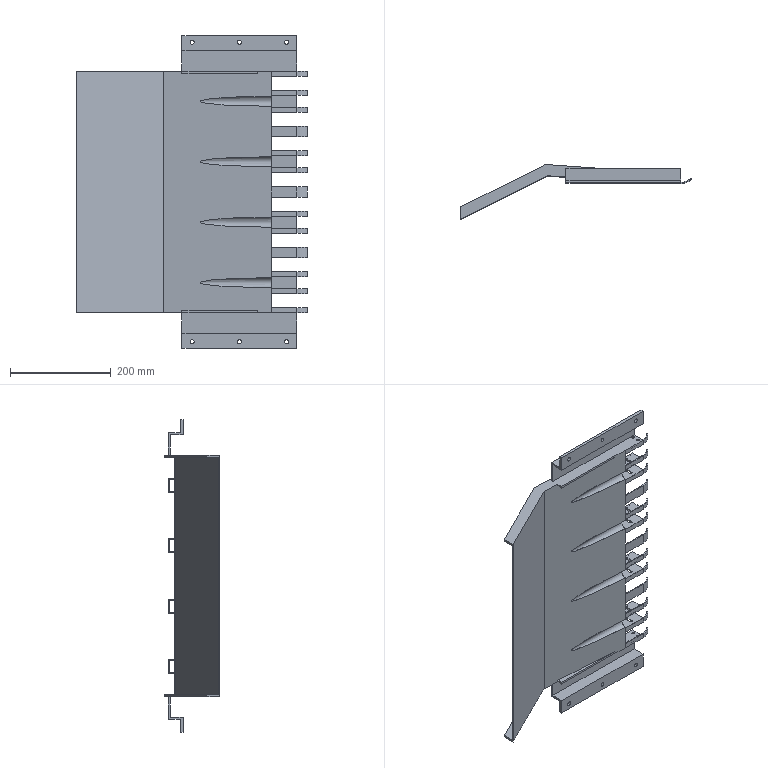Part | SolidWorks | features BaseBody 1 | 1 solid | 239 faces | box 457.67 x 108.321 x 620 mm | volume 727170 mm3 | plane 152 | cylinder 87 | commonest cylinder face diameters 7 x24 5 x16 55.99 x13 60 x13 8 x12 20 x4